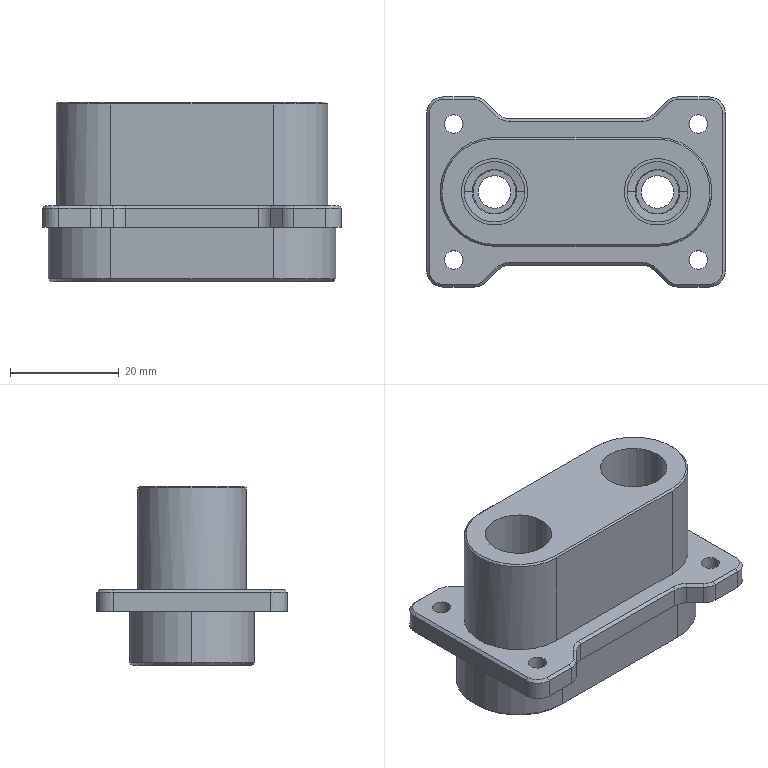Part | 1 solid | 116 faces | box 55 x 35 x 33 mm | volume 28334 mm3 | cylinder 46 | plane 40 | cone 30 | commonest cylinder face diameters 6 x16 3.4 x8 8.17 x4 11.15 x4 11.8 x4 12.25 x4